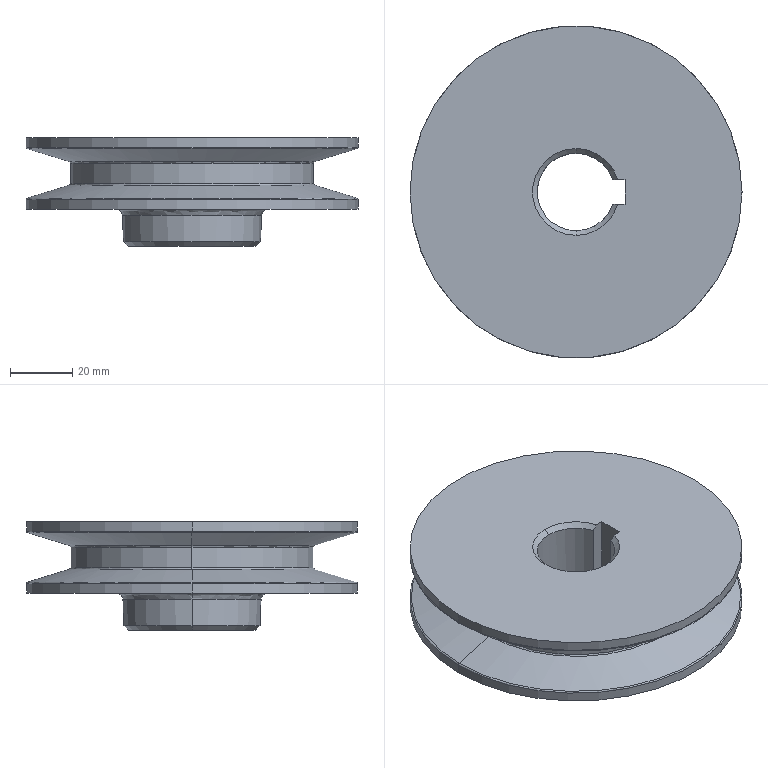Part | SolidWorks | features BaseBody 1 | 1 solid | 37 faces | box 107 x 107 x 35 mm | volume 157181 mm3 | cone 13 | spline 10 | cylinder 8 | plane 6 | commonest cylinder face diameters 107 x4 25 x2 78.4 x2